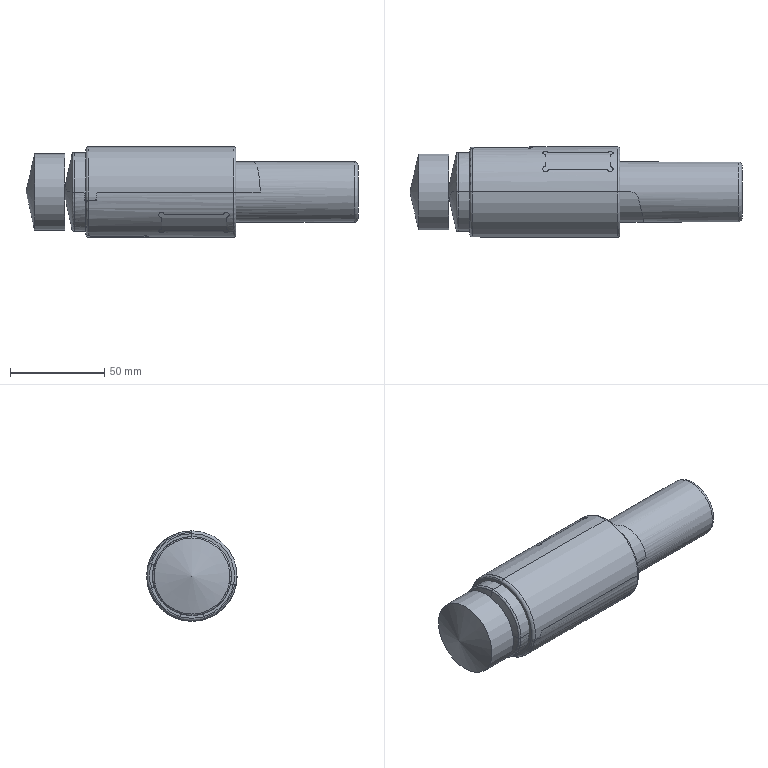NC program | NX | posted with a generic post | part box 176.413 x 48 x 48 mm
Lines 1 to 1741 of 71815:
N10 G17 G21 G94 G90
(FLOOR_WALL , TOOL : D16R0.8)
N12 T16 M6
N14 G54
N16 G17 G0 G90 X-98.197 Y-17.836 S2000 M3
N18 G43 Z30.115 H16
N20 Z24.006
N22 G94 G1 Z22.506 F1000.
N24 X-103.22 Y-9.136
N26 G3 X-104.606 Y-8.336 R1.6
N28 G1 X-143.133 F2000.
N30 G2 X-143.615 Y-8.1 R0.67
N32 G1 X-65.61
N34 X-65.895 Y-8.32
N36 X-66. Y-8.336
N38 X-104.606
N40 G3 X-105.992 Y-9.136 R1.6
N42 G1 X-111.015 Y-17.836
N44 Z24.006
N46 G0 X-98.223 Y-18.479 Z23.757
N48 G1 Z22.257 F1000.
N50 X-103.246 Y-9.779
N52 G3 X-104.632 Y-8.979 R1.6
N54 G1 X-143.142 F2000.
N56 G2 X-144.048 Y-8.1 R1.265
N58 G1 X-65.276
N60 X-65.559 Y-8.702
N62 X-65.618 Y-8.774
N64 X-65.768 Y-8.906
N66 X-65.905 Y-8.967
N68 X-66. Y-8.979
N70 X-104.632
N72 G3 X-106.017 Y-9.779 R1.6
N74 G1 X-111.04 Y-18.479
N76 Z23.757
N78 G0 X-98.843 Y-19.073 Z23.508
N80 G1 Z22.008 F1000.
N82 X-103.866 Y-10.373
N84 G3 X-105.252 Y-9.573 R1.6
N86 G1 X-143.133 F2000.
N88 X-143.218 Y-9.567
N90 X-143.587 Y-9.395
N92 X-143.969 Y-8.916
N94 X-144.131 Y-8.575
N96 X-144.292 Y-8.1
N98 X-65.088
N100 G2 X-65.494 Y-9.248 R3.11
N102 G1 X-65.705 Y-9.461
N104 X-65.842 Y-9.541
N106 X-65.98 Y-9.573
N108 X-105.252
N110 G3 X-106.638 Y-10.373 R1.6
N112 G1 X-111.661 Y-19.073
N114 Z23.508
N116 G0 X-99.004 Y-19.626 Z23.259
N118 G1 Z21.759 F1000.
N120 X-104.027 Y-10.926
N122 G3 X-105.413 Y-10.126 R1.6
N124 G1 X-143.156 F2000.
N126 G2 X-143.924 Y-9.579 R1.015
N128 G1 X-144.104 Y-9.249
N130 X-144.259 Y-8.852
N132 X-144.447 Y-8.1
N134 X-65.
N136 G2 X-65.352 Y-9.578 R4.236
N138 X-66. Y-10.126 R0.876
N140 G1 X-105.413
N142 G3 X-106.798 Y-10.926 R1.6
N144 G1 X-111.821 Y-19.626
N146 Z23.259
N148 G0 X-99.265 Y-20.145 Z23.01
N150 G1 Z21.51 F1000.
N152 X-104.288 Y-11.445
N154 G3 X-105.674 Y-10.645 R1.6
N156 G1 X-143.133 F2000.
N158 X-143.313 Y-10.62
N160 X-143.589 Y-10.484
N162 X-143.774 Y-10.316
N164 G2 X-144.546 Y-8.1 R4.023
N166 G1 X-64.999
N168 X-65.027 Y-8.901
N170 G2 X-65.333 Y-10.089 R3.297
N172 G1 X-65.705 Y-10.544
N174 X-66. Y-10.645
N176 X-105.674
N178 G3 X-107.059 Y-11.445 R1.6
N180 G1 X-112.082 Y-20.145
N182 Z23.01
N184 G0 X-98.654 Y-20.634 Z22.761
N186 G1 Z21.261 F1000.
N188 X-103.677 Y-11.934
N190 G3 X-105.063 Y-11.134 R1.6
N192 G1 X-143.133 F2000.
N194 G2 X-144.126 Y-10.298 R1.212
N196 G1 X-144.302 Y-9.879
N198 G2 X-144.631 Y-8.1 R6.287
N200 G1 X-65.
N202 X-65.03 Y-9.501
N204 G2 X-65.367 Y-10.657 R2.686
N206 G1 X-65.72 Y-11.048
N208 X-66. Y-11.134
N210 X-105.063
N212 G3 X-106.448 Y-11.934 R1.6
N214 G1 X-111.471 Y-20.634
N216 Z22.761
N218 G0 X-98.554 Y-21.097 Z22.512
N220 G1 Z21.012 F1000.
N222 X-103.577 Y-12.397
N224 G3 X-104.963 Y-11.597 R1.6
N226 G1 X-143.133 F2000.
N228 G2 X-144.092 Y-10.862 R1.1
N230 G1 X-144.31 Y-10.391
N232 G2 X-144.633 Y-8.206 R6.418
N234 G1 Y-8.1
N236 X-65.
N238 Y-8.935
N240 X-64.999 Y-9.628
N242 G2 X-65.276 Y-10.985 R3.254
N244 X-65.93 Y-11.592 R1.015
N246 G1 X-66. Y-11.597
N248 X-104.963
N250 G3 X-106.348 Y-12.397 R1.6
N252 G1 X-111.371 Y-21.097
N254 Z22.512
N256 G0 X-100.012 Y-21.537 Z22.263
N258 G1 Z20.763 F1000.
N260 X-105.035 Y-12.837
N262 G3 X-106.42 Y-12.037 R1.6
N264 G1 X-143.187 Y-12.035 F2000.
N266 G2 X-144.11 Y-11.299 R1.22
N268 G1 X-144.328 Y-10.831
N270 G2 X-144.57 Y-9.816 R6.02
N272 G1 X-144.823 Y-8.1
N274 X-65.
N276 Y-9.765
N278 Y-10.121
N280 G2 X-65.33 Y-11.539 R3.11
N282 G1 X-65.696 Y-11.942
N284 X-66. Y-12.037
N286 X-106.42
N288 G3 X-107.806 Y-12.837 R1.6
N290 G1 X-112.829 Y-21.537
N292 Z22.263
N294 G0 X-97.913 Y-21.956 Z22.014
N296 G1 Z20.514 F1000.
N298 X-102.936 Y-13.256
N300 G3 X-104.322 Y-12.456 R1.6
N302 G1 X-143.301 F2000.
N304 G2 X-143.56 Y-12.363 R0.818
N306 G1 X-143.863 Y-12.087
N308 X-144.058 Y-11.83
N310 X-144.287 Y-11.403
N312 G2 X-144.509 Y-10.656 R5.376
N314 G1 X-145.07 Y-8.1
N316 X-65.
N318 X-65.019 Y-10.828
N320 X-65.106 Y-11.423
N322 G2 X-65.442 Y-12.144 R1.812
N324 G1 X-65.802 Y-12.418
N326 X-65.96 Y-12.455
N328 X-104.322 Y-12.456
N330 G3 X-105.707 Y-13.256 R1.6
N332 G1 X-110.73 Y-21.956
N334 Z22.014
N336 G0 X-100.502 Y-22.357 Z21.765
N338 G1 Z20.265 F1000.
N340 X-105.525 Y-13.657
N342 G3 X-106.91 Y-12.857 R1.6
N344 G1 X-143.159 F2000.
N346 G2 X-144.09 Y-12.202 R1.193
N348 G1 X-144.316 Y-11.769
N350 G2 X-144.456 Y-11.33 R5.168
N352 G1 X-145.325 Y-8.1
N354 X-65.
N356 Y-10.582
N358 X-64.998 Y-11.043
N360 G2 X-65.345 Y-12.421 R2.704
N362 G1 X-65.542 Y-12.649
N364 X-65.693 Y-12.767
N366 X-66. Y-12.857
N368 X-106.91
N370 G3 X-108.296 Y-13.657 R1.6
N372 G1 X-113.319 Y-22.357
N374 Z21.765
N376 G0 X-100.642 Y-22.742 Z21.516
N378 G1 Z20.016 F1000.
N380 X-105.665 Y-14.042
N382 G3 X-107.051 Y-13.242 R1.6
N384 G1 X-143.133 F2000.
N386 G2 X-144.023 Y-12.704 R1.1
N388 G1 X-144.269 Y-12.31
N390 G2 X-144.441 Y-11.862 R4.065
N392 G1 X-145.637 Y-8.1
N394 X-65.
N396 X-64.998 Y-11.043
N398 X-65. Y-11.226
N400 Y-11.506
N402 G2 X-65.249 Y-12.648 R2.895
N404 G1 X-65.454 Y-12.945
N406 X-65.604 Y-13.093
N408 X-65.941 Y-13.239
N410 X-66. Y-13.242
N412 X-107.051
N414 G3 X-108.437 Y-14.042 R1.6
N416 G1 X-113.46 Y-22.742
N418 Z21.516
N420 G0 X-101.061 Y-23.111 Z21.267
N422 G1 Z19.767 F1000.
N424 X-106.084 Y-14.411
N426 G3 X-107.469 Y-13.611 R1.6
N428 G1 X-143.133 F2000.
N430 G2 X-144.197 Y-12.84 R1.247
N432 X-144.407 Y-12.353 R3.996
N434 G1 X-145.911 Y-8.1
N436 X-65.
N438 X-65.03 Y-12.224
N440 X-65.133 Y-12.767
N442 G2 X-65.457 Y-13.363 R1.509
N444 G1 X-65.855 Y-13.592
N446 X-66. Y-13.611
N448 X-107.469
N450 G3 X-108.855 Y-14.411 R1.6
N452 G1 X-113.878 Y-23.111
N454 Z21.267
N456 G0 X-101.143 Y-23.465 Z21.019
N458 G1 Z19.519 F1000.
N460 X-106.166 Y-14.765
N462 G3 X-107.552 Y-13.965 R1.6
N464 G1 X-143.133 F2000.
N466 X-143.345 Y-13.939
N468 X-143.718 Y-13.76
N470 X-143.92 Y-13.578
N472 X-144.118 Y-13.322
N474 X-144.359 Y-12.876
N476 X-146.143 Y-8.137
N478 X-146.598 Y-8.1
N480 X-65.
N482 X-65.032 Y-12.714
N484 G2 X-65.321 Y-13.545 R1.971
N486 G1 X-65.575 Y-13.802
N488 X-65.637 Y-13.847
N490 X-66. Y-13.965
N492 X-107.552
N494 G3 X-108.937 Y-14.765 R1.6
N496 G1 X-113.96 Y-23.465
N498 Z21.019
N500 G0 X-98.202 Y-23.807 Z20.77
N502 G1 Z19.27 F1000.
N504 X-103.225 Y-15.107
N506 G3 X-104.611 Y-14.307 R1.6
N508 G1 X-143.133 F2000.
N510 G2 X-144.167 Y-13.629 R1.292
N512 X-144.361 Y-13.235 R3.566
N514 G1 X-146.294 Y-8.597
N516 X-147.856 Y-8.512
N518 Y-8.1
N520 X-65.
N522 X-65.026 Y-12.971
N524 G2 X-65.637 Y-14.192 R1.633
N526 G1 X-66. Y-14.307
N528 X-104.611
N530 G3 X-105.997 Y-15.107 R1.6
N532 G1 X-111.02 Y-23.807
N534 Z20.77
N536 G0 X-101.11 Y-24.136 Z20.521
N538 G1 Z19.021 F1000.
N540 X-106.133 Y-15.436
N542 G3 X-107.518 Y-14.636 R1.6
N544 G1 X-143.133 F2000.
N546 G2 X-144.099 Y-14.051 R1.197
N548 G1 X-144.353 Y-13.627
N550 X-146.38 Y-9.003
N552 X-147.856 Y-8.969
N554 Y-8.1
N556 X-65.
N558 X-65.032 Y-13.457
N560 G2 X-65.321 Y-14.237 R1.791
N562 G1 X-65.578 Y-14.483
N564 X-65.651 Y-14.533
N566 X-66. Y-14.636
N568 X-107.518
N570 G3 X-108.904 Y-15.436 R1.6
N572 G1 X-113.927 Y-24.136
N574 Z20.521
N576 G0 X-97.817 Y-24.454 Z20.272
N578 G1 Z18.772 F1000.
N580 X-102.84 Y-15.754
N582 G3 X-104.225 Y-14.954 R1.6
N584 G1 X-143.133 F2000.
N586 G2 X-144.127 Y-14.342 R1.2
N588 G1 X-144.406 Y-13.858
N590 X-146.44 Y-9.44
N592 X-147.856 Y-9.432
N594 Y-8.1
N596 X-65.
N598 X-65.023 Y-13.658
N600 G2 X-65.653 Y-14.854 R1.529
N602 G1 X-66. Y-14.954
N604 X-104.225
N606 G3 X-105.611 Y-15.754 R1.6
N608 G1 X-110.634 Y-24.454
N610 Z20.272
N612 G0 X-100.993 Y-24.761 Z20.023
N614 G1 Z18.523 F1000.
N616 X-106.016 Y-16.061
N618 G3 X-107.402 Y-15.261 R1.6
N620 G1 X-143.206 Y-15.259 F2000.
N622 X-143.668 Y-15.106
N624 X-143.877 Y-14.949
N626 X-144.07 Y-14.739
N628 X-144.335 Y-14.334
N630 X-146.479 Y-9.895
N632 X-147.856
N634 Y-8.1
N636 X-65.
N638 X-65.023 Y-14.113
N640 G2 X-65.292 Y-14.835 R1.815
N642 G1 X-65.542 Y-15.087
N644 X-65.622 Y-15.145
N646 X-65.803 Y-15.23
N648 X-65.977 Y-15.261
N650 X-107.402
N652 G3 X-108.788 Y-16.061 R1.6
N654 G1 X-113.81 Y-24.761
N656 Z20.023
N658 G0 X-97.282 Y-25.059 Z19.774
N660 G1 Z18.274 F1000.
N662 X-102.304 Y-16.359
N664 G3 X-103.69 Y-15.559 R1.6
N666 G1 X-143.133 F2000.
N668 X-143.241 Y-15.553
N670 X-143.458 Y-15.504
N672 X-143.56 Y-15.463
N674 X-144.009 Y-15.12
N676 X-144.305 Y-14.718
N678 X-146.411 Y-10.549
N680 X-147.856 Y-10.484
N682 Y-8.1
N684 X-65.
N686 X-65.023 Y-14.315
N688 G2 X-65.68 Y-15.477 R1.424
N690 G1 X-66. Y-15.559
N692 X-103.69
N694 G3 X-105.076 Y-16.359 R1.6
N696 G1 X-110.099 Y-25.059
N698 Z19.774
N700 G0 X-97.018 Y-25.346 Z19.525
N702 G1 Z18.025 F1000.
N704 X-102.041 Y-16.646
N706 G3 X-103.427 Y-15.846 R1.6
N708 G1 X-143.133 F2000.
N710 G2 X-144.236 Y-15.139 R1.354
N712 G1 X-144.29 Y-15.04
N714 X-146.368 Y-11.084
N716 X-147.856 Y-10.982
N718 Y-8.1
N720 X-65.
N722 Y-14.287
N724 G2 X-65.611 Y-15.727 R1.652
N726 G1 X-65.684 Y-15.769
N728 X-65.843 Y-15.828
N730 X-66. Y-15.846
N732 X-103.427
N734 G3 X-104.813 Y-16.646 R1.6
N736 G1 X-109.836 Y-25.346
N738 Z19.525
N740 G0 X-100.846 Y-25.625 Z19.276
N742 G1 Z17.776 F1000.
N744 X-105.869 Y-16.925
N746 G3 X-107.255 Y-16.125 R1.6
N748 G1 X-143.133 F2000.
N750 G2 X-144.16 Y-15.514 R1.268
N752 G1 X-146.715 Y-11.181
N754 X-147.856
N756 Y-8.1
N758 X-65.
N760 Y-14.556
N762 Y-14.757
N764 G2 X-65.26 Y-15.676 R1.72
N766 G1 X-65.514 Y-15.937
N768 X-65.6 Y-16.
N770 X-65.765 Y-16.084
N772 X-65.943 Y-16.123
N774 X-107.255 Y-16.125
N776 G3 X-108.64 Y-16.925 R1.6
N778 G1 X-113.663 Y-25.625
N780 Z19.276
N782 G0 X-96.821 Y-25.895 Z19.027
N784 G1 Z17.527 F1000.
N786 X-101.844 Y-17.195
N788 G3 X-103.23 Y-16.395 R1.6
N790 G1 X-143.133 F2000.
N792 G2 X-144.315 Y-15.589 R1.416
N794 G1 X-146.577 Y-11.568
N796 X-147.856
N798 Y-8.1
N800 X-65.
N802 X-65.023 Y-15.218
N804 G2 X-65.879 Y-16.385 R1.309
N806 G1 X-66. Y-16.395
N808 X-103.23
N810 G3 X-104.616 Y-17.195 R1.6
N812 G1 X-109.639 Y-25.895
N814 Z19.027
N816 G0 X-96.475 Y-26.158 Z18.778
N818 G1 Z17.278 F1000.
N820 X-101.498 Y-17.458
N822 G3 X-102.884 Y-16.658 R1.6
N824 G1 X-143.145 Y-16.657 F2000.
N826 G2 X-144.078 Y-16.172 R1.219
N828 G1 X-144.395 Y-15.724
N830 X-146.402 Y-12.223
N832 X-147.856 Y-12.13
N834 Y-8.1
N836 X-65.
N838 Y-15.181
N840 G2 X-65.824 Y-16.635 R1.414
N842 G1 X-66. Y-16.658
N844 X-102.884
N846 G3 X-104.27 Y-17.458 R1.6
N848 G1 X-109.293 Y-26.158
N850 Z18.778
N852 G0 X-96.479 Y-26.412 Z18.529
N854 G1 Z17.029 F1000.
N856 X-101.502 Y-17.712
N858 G3 X-102.888 Y-16.912 R1.6
N860 G1 X-143.133 F2000.
N862 X-143.283 Y-16.901
N864 X-143.776 Y-16.706
N866 X-143.986 Y-16.532
N868 X-144.295 Y-16.166
N870 X-146.598 Y-12.289
N872 X-147.856
N874 Y-8.1
N876 X-65.
N878 Y-15.46
N880 G2 X-65.753 Y-16.868 R1.47
N882 G1 X-65.935 Y-16.909
N884 X-66. Y-16.912
N886 X-102.888
N888 G3 X-104.274 Y-17.712 R1.6
N890 G1 X-109.297 Y-26.412
N892 Z18.529
N894 G0 X-96.414 Y-26.659 Z18.28
N896 G1 Z16.78 F1000.
N898 X-101.437 Y-17.959
N900 G3 X-102.823 Y-17.159 R1.6
N902 G1 X-143.133 F2000.
N904 X-143.362 Y-17.134
N906 X-143.813 Y-16.931
N908 X-143.887 Y-16.874
N910 X-144.089 Y-16.674
N912 X-146.958 Y-12.627
N914 X-147.856
N916 Y-8.1
N918 X-65.
N920 Y-15.73
N922 X-65.022 Y-16.036
N924 X-65.078 Y-16.292
N926 X-65.174 Y-16.542
N928 X-65.517 Y-16.985
N930 X-65.87 Y-17.147
N932 X-66. Y-17.159
N934 X-102.823
N936 G3 X-104.209 Y-17.959 R1.6
N938 G1 X-109.232 Y-26.659
N940 Z18.28
N942 G0 X-96.072 Y-26.899 Z18.031
N944 G1 Z16.531 F1000.
N946 X-101.095 Y-18.199
N948 G3 X-102.481 Y-17.399 R1.6
N950 G1 X-143.198 Y-17.397 F2000.
N952 X-143.428 Y-17.359
N954 X-143.561 Y-17.313
N956 X-143.999 Y-17.017
N958 X-144.31 Y-16.651
N960 X-146.507 Y-13.102
N962 X-147.856 Y-13.056
N964 Y-8.1
N966 X-65.
N968 Y-15.991
N970 G2 X-65.822 Y-17.377 R1.388
N972 G1 X-66. Y-17.399
N974 X-102.481
N976 G3 X-103.866 Y-18.199 R1.6
N978 G1 X-108.889 Y-26.899
N980 Z18.031
N982 G0 X-96.078 Y-27.132 Z17.782
N984 G1 Z16.282 F1000.
N986 X-101.101 Y-18.432
N988 G3 X-102.487 Y-17.632 R1.6
N990 G1 X-143.133 F2000.
N992 X-143.307 Y-17.618
N994 X-143.536 Y-17.557
N996 X-143.66 Y-17.502
N998 X-144.112 Y-17.134
N1000 X-146.846 Y-13.262
N1002 X-147.856
N1004 Y-8.1
N1006 X-65.
N1008 Y-16.245
N1010 G2 X-65.761 Y-17.593 R1.367
N1012 G1 X-65.948 Y-17.63
N1014 X-102.487 Y-17.632
N1016 G3 X-103.872 Y-18.432 R1.6
N1018 G1 X-108.895 Y-27.132
N1020 Z17.782
N1022 G0 X-95.773 Y-27.359 Z17.533
N1024 G1 Z16.033 F1000.
N1026 X-100.796 Y-18.659
N1028 G3 X-102.182 Y-17.859 R1.6
N1030 G1 X-143.309 Y-17.845 F2000.
N1032 G2 X-144.245 Y-17.19 R1.386
N1034 G1 X-146.243 Y-13.562
N1036 X-147.856
N1038 Y-8.1
N1040 X-65.
N1042 Y-16.491
N1044 X-65.022 Y-16.783
N1046 X-65.095 Y-17.079
N1048 X-65.198 Y-17.315
N1050 X-65.546 Y-17.712
N1052 X-65.872 Y-17.848
N1054 X-66. Y-17.859
N1056 X-102.182
N1058 G3 X-103.568 Y-18.659 R1.6
N1060 G1 X-108.591 Y-27.359
N1062 Z17.533
N1064 G0 X-95.813 Y-27.579 Z17.284
N1066 G1 Z15.784 F1000.
N1068 X-100.836 Y-18.879
N1070 G3 X-102.221 Y-18.079 R1.6
N1072 G1 X-143.133 F2000.
N1074 X-143.259 Y-18.072
N1076 X-143.686 Y-17.939
N1078 X-143.905 Y-17.794
N1080 X-144.096 Y-17.612
N1082 X-146.903 Y-13.851
N1084 X-147.856
N1086 Y-8.1
N1088 X-65.
N1090 Y-16.729
N1092 G2 X-66. Y-18.079 R1.22
N1094 G1 X-102.221
N1096 G3 X-103.607 Y-18.879 R1.6
N1098 G1 X-108.63 Y-27.579
N1100 Z17.284
N1102 G0 X-95.577 Y-27.794 Z17.035
N1104 G1 Z15.535 F1000.
N1106 X-100.6 Y-19.094
N1108 G3 X-101.986 Y-18.294 R1.6
N1110 G1 X-143.133 F2000.
N1112 X-143.368 Y-18.269
N1114 X-143.765 Y-18.11
N1116 X-143.98 Y-17.948
N1118 X-144.171 Y-17.743
N1120 X-146.55 Y-14.13
N1122 X-147.856
N1124 Y-8.1
N1126 X-65.
N1128 Y-16.96
N1130 G2 X-65.975 Y-18.293 R1.185
N1132 G1 X-101.986 Y-18.294
N1134 G3 X-103.372 Y-19.094 R1.6
N1136 G1 X-108.395 Y-27.794
N1138 Z17.035
N1140 G0 X-95.362 Y-28.002 Z16.786
N1142 G1 Z15.286 F1000.
N1144 X-100.385 Y-19.302
N1146 G3 X-101.771 Y-18.502 R1.6
N1148 G1 X-143.133 F2000.
N1150 X-143.371 Y-18.478
N1152 X-143.849 Y-18.266
N1154 X-144.059 Y-18.086
N1156 X-144.246 Y-17.856
N1158 X-146.226 Y-14.399
N1160 X-147.856
N1162 Y-8.1
N1164 X-65.
N1166 Y-17.185
N1168 G2 X-66. Y-18.502 R1.188
N1170 G1 X-101.771
N1172 G3 X-103.157 Y-19.302 R1.6
N1174 G1 X-108.179 Y-28.002
N1176 Z16.786
N1178 G0 X-95.354 Y-28.205 Z16.537
N1180 G1 Z15.037 F1000.
N1182 X-100.377 Y-19.505
N1184 G3 X-101.763 Y-18.705 R1.6
N1186 G1 X-143.158 F2000.
N1188 X-143.397 Y-18.675
N1190 X-143.937 Y-18.405
N1192 X-144.139 Y-18.206
N1194 X-146.663 Y-14.659
N1196 X-147.856
N1198 Y-8.1
N1200 X-65.
N1202 X-65.023 Y-17.686
N1204 G2 X-66. Y-18.705 R1.05
N1206 G1 X-101.763
N1208 G3 X-103.149 Y-19.505 R1.6
N1210 G1 X-108.172 Y-28.205
N1212 Z16.537
N1214 G0 X-95.133 Y-28.403 Z16.288
N1216 G1 Z14.788 F1000.
N1218 X-100.156 Y-19.703
N1220 G3 X-101.541 Y-18.903 R1.6
N1222 G1 X-143.202 Y-18.9 F2000.
N1224 X-143.441 Y-18.862
N1226 X-143.595 Y-18.81
N1228 X-144.027 Y-18.526
N1230 X-144.219 Y-18.308
N1232 X-146.299 Y-14.91
N1234 X-147.856
N1236 Y-8.1
N1238 X-65.
N1240 X-65.023 Y-17.892
N1242 G2 X-66. Y-18.903 R1.093
N1244 G1 X-101.541
N1246 G3 X-102.927 Y-19.703 R1.6
N1248 G1 X-107.95 Y-28.403
N1250 Z16.288
N1252 G0 X-95.145 Y-28.595 Z16.039
N1254 G1 Z14.539 F1000.
N1256 X-100.168 Y-19.895
N1258 G3 X-101.553 Y-19.095 R1.6
N1260 G1 X-143.133 F2000.
N1262 X-143.373 Y-19.07
N1264 X-143.781 Y-18.909
N1266 X-143.996 Y-18.75
N1268 X-144.118 Y-18.629
N1270 X-146.758 Y-15.153
N1272 X-147.856
N1274 Y-8.1
N1276 X-65.
N1278 Y-17.821
N1280 G2 X-65.964 Y-19.094 R1.158
N1282 G1 X-101.553 Y-19.095
N1284 G3 X-102.939 Y-19.895 R1.6
N1286 G1 X-107.962 Y-28.595
N1288 Z16.039
N1290 G0 X-95.06 Y-28.782 Z15.79
N1292 G1 Z14.29 F1000.
N1294 X-100.083 Y-20.082
N1296 G3 X-101.469 Y-19.282 R1.6
N1298 G1 X-143.133 F2000.
N1300 G2 X-144.098 Y-18.842 R1.319
N1302 G1 X-146.85 Y-15.388
N1304 X-147.856
N1306 Y-8.1
N1308 X-65.
N1310 Y-18.022
N1312 G2 X-66. Y-19.282 R1.158
N1314 G1 X-101.469
N1316 G3 X-102.854 Y-20.082 R1.6
N1318 G1 X-107.877 Y-28.782
N1320 Z15.79
N1322 G0 X-94.913 Y-28.964 Z15.541
N1324 G1 Z14.041 F1000.
N1326 X-99.936 Y-20.264
N1328 G3 X-101.322 Y-19.464 R1.6
N1330 G1 X-143.174 Y-19.463 F2000.
N1332 G2 X-144.123 Y-19.002 R1.338
N1334 G1 X-146.728 Y-15.615
N1336 X-147.856
N1338 Y-8.1
N1340 X-65.
N1342 Y-18.216
N1344 G2 X-66. Y-19.464 R1.134
N1346 G1 X-101.322
N1348 G3 X-102.707 Y-20.264 R1.6
N1350 G1 X-107.73 Y-28.964
N1352 Z15.541
N1354 G0 X-94.765 Y-29.141 Z15.293
N1356 G1 Z13.793 F1000.
N1358 X-99.788 Y-20.441
N1360 G3 X-101.173 Y-19.641 R1.6
N1362 G1 X-143.133 F2000.
N1364 G2 X-144.156 Y-19.146 R1.352
N1366 G1 X-146.572 Y-15.836
N1368 X-147.856
N1370 Y-8.1
N1372 X-62.231
N1374 X-62.229 Y-8.11
N1376 X-65.
N1378 Y-18.406
N1380 G2 X-66. Y-19.641 R1.133
N1382 G1 X-101.173
N1384 G3 X-102.559 Y-20.441 R1.6
N1386 G1 X-107.582 Y-29.141
N1388 Z15.293
N1390 G0 X-94.8 Y-29.313 Z15.044
N1392 G1 Z13.544 F1000.
N1394 X-99.823 Y-20.613
N1396 G3 X-101.209 Y-19.813 R1.6
N1398 G1 X-143.133 F2000.
N1400 X-143.378 Y-19.789
N1402 X-143.807 Y-19.619
N1404 X-144.024 Y-19.457
N1406 X-144.21 Y-19.259
N1408 X-146.342 Y-16.049
N1410 X-147.856
N1412 Y-8.1
N1414 X-62.231
N1416 X-62.131 Y-8.519
N1418 X-65.
N1420 Y-18.59
N1422 G2 X-66. Y-19.813 R1.154
N1424 G1 X-101.209
N1426 G3 X-102.595 Y-20.613 R1.6
N1428 G1 X-107.618 Y-29.313
N1430 Z15.044
N1432 G0 X-95.063 Y-29.481 Z14.795
N1434 G1 Z13.295 F1000.
N1436 X-100.086 Y-20.781
N1438 G3 X-101.472 Y-19.981 R1.6
N1440 G1 X-143.133 F2000.
N1442 X-143.379 Y-19.957
N1444 X-143.871 Y-19.748
N1446 X-144.083 Y-19.573
N1448 X-146.909 Y-16.256
N1450 X-147.856
N1452 Y-8.1
N1454 X-62.231
N1456 X-62.038 Y-8.902
N1458 X-65.
N1460 X-65.001 Y-18.818
N1462 G2 X-66. Y-19.981 R1.129
N1464 G1 X-101.472
N1466 G3 X-102.858 Y-20.781 R1.6
N1468 G1 X-107.88 Y-29.481
N1470 Z14.795
N1472 G0 X-95.057 Y-29.645 Z14.546
N1474 G1 Z13.046 F1000.
N1476 X-100.08 Y-20.945
N1478 G3 X-101.466 Y-20.145 R1.6
N1480 G1 X-143.212 Y-20.142 F2000.
N1482 G2 X-144.142 Y-19.678 R1.373
N1484 G1 X-146.622 Y-16.456
N1486 X-147.856
N1488 Y-8.1
N1490 X-62.231
N1492 X-61.951 Y-9.263
N1494 X-65.
N1496 X-65.024 Y-19.205
N1498 G2 X-66. Y-20.145 R1.059
N1500 G1 X-101.466
N1502 G3 X-102.851 Y-20.945 R1.6
N1504 G1 X-107.874 Y-29.645
N1506 Z14.546
N1508 G0 X-95.055 Y-29.804 Z14.297
N1510 G1 Z12.797 F1000.
N1512 X-100.078 Y-21.104
N1514 G3 X-101.463 Y-20.304 R1.6
N1516 G1 X-143.133 F2000.
N1518 G2 X-144.203 Y-19.772 R1.383
N1520 G1 X-146.354 Y-16.651
N1522 X-147.856
N1524 Y-8.1
N1526 X-62.231
N1528 X-61.869 Y-9.604
N1530 X-65.
N1532 Y-19.111
N1534 G2 X-66. Y-20.304 R1.124
N1536 G1 X-101.463
N1538 G3 X-102.849 Y-21.104 R1.6
N1540 G1 X-107.872 Y-29.804
N1542 Z14.297
N1544 G0 X-95.297 Y-29.959 Z14.048
N1546 G1 Z12.548 F1000.
N1548 X-100.32 Y-21.259
N1550 G3 X-101.706 Y-20.459 R1.6
N1552 G1 X-143.133 F2000.
N1554 G2 X-144.075 Y-20.067 R1.358
N1556 G1 X-146.914 Y-16.839
N1558 X-147.856
N1560 Y-8.1
N1562 X-62.231
N1564 X-61.792 Y-9.927
N1566 X-65.
N1568 Y-19.276
N1570 G2 X-66. Y-20.459 R1.086
N1572 G1 X-101.706
N1574 G3 X-103.092 Y-21.259 R1.6
N1576 G1 X-108.115 Y-29.959
N1578 Z14.048
N1580 G0 X-95.258 Y-30.109 Z13.799
N1582 G1 Z12.299 F1000.
N1584 X-100.281 Y-21.409
N1586 G3 X-101.667 Y-20.609 R1.6
N1588 G1 X-143.133 F2000.
N1590 G2 X-144.147 Y-20.149 R1.382
N1592 G1 X-146.586 Y-17.022
N1594 X-147.856
N1596 Y-8.1
N1598 X-62.231
N1600 X-61.718 Y-10.234
N1602 X-65.
N1604 Y-19.436
N1606 G2 X-65.966 Y-20.609 R1.091
N1608 G1 X-101.667
N1610 G3 X-103.052 Y-21.409 R1.6
N1612 G1 X-108.075 Y-30.109
N1614 Z13.799
N1616 G0 X-95.23 Y-30.256 Z13.55
N1618 G1 Z12.05 F1000.
N1620 X-100.253 Y-21.556
N1622 G3 X-101.638 Y-20.756 R1.6
N1624 G1 X-143.133 F2000.
N1626 G2 X-144.218 Y-20.217 R1.4
N1628 G1 X-146.286 Y-17.199
N1630 X-147.856
N1632 Y-8.1
N1634 X-62.231
N1636 X-61.648 Y-10.526
N1638 X-65.
N1640 Y-19.591
N1642 G2 X-66. Y-20.756 R1.088
N1644 G1 X-101.638
N1646 G3 X-103.024 Y-21.556 R1.6
N1648 G1 X-108.047 Y-30.256
N1650 Z13.55
N1652 G0 X-95.357 Y-30.398 Z13.301
N1654 G1 Z11.801 F1000.
N1656 X-100.38 Y-21.698
N1658 G3 X-101.766 Y-20.898 R1.6
N1660 G1 X-143.133 F2000.
N1662 G2 X-144.158 Y-20.432 R1.389
N1664 G1 X-146.53 Y-17.371
N1666 X-147.856
N1668 Y-8.102
N1670 X-62.231
N1672 X-61.581 Y-10.805
N1674 X-65.
N1676 Y-19.742
N1678 G2 X-66. Y-20.898 R1.106
N1680 G1 X-101.766
N1682 G3 X-103.152 Y-21.698 R1.6
N1684 G1 X-108.175 Y-30.398
N1686 Z13.301
N1688 G0 X-95.386 Y-30.537 Z13.052
N1690 G1 Z11.552 F1000.
N1692 X-100.409 Y-21.837
N1694 G3 X-101.795 Y-21.037 R1.6
N1696 G1 X-143.133 F2000.
N1698 G2 X-144.176 Y-20.555 R1.398
N1700 G1 X-146.454 Y-17.537
N1702 X-147.856
N1704 Y-8.108
N1706 X-62.229
N1708 X-61.517 Y-11.07
N1710 X-65.
N1712 Y-19.889
N1714 G2 X-66. Y-21.037 R1.102
N1716 G1 X-101.795
N1718 G3 X-103.181 Y-21.837 R1.6
N1720 G1 X-108.204 Y-30.537
N1722 Z13.052
N1724 G0 X-95.408 Y-30.672 Z12.803
N1726 G1 Z11.303 F1000.
N1728 X-100.431 Y-21.972
N1730 G3 X-101.816 Y-21.172 R1.6
N1732 G1 X-143.133 F2000.
N1734 G2 X-144.198 Y-20.668 R1.401
N1736 G1 X-146.362 Y-17.699
N1738 X-147.856
N1740 Y-8.12
N1742 X-62.226
N1744 X-61.456 Y-11.324
N1746 X-65.
N1748 Y-20.031
N1750 G2 X-66. Y-21.172 R1.099
N1752 G1 X-101.816
N1754 G3 X-103.202 Y-21.972 R1.6
N1756 G1 X-108.225 Y-30.672
N1758 Z12.803
N1760 G0 X-95.669 Y-30.803 Z12.554
N1762 G1 Z11.054 F1000.
N1764 X-100.692 Y-22.103
N1766 G3 X-102.078 Y-21.303 R1.6
N1768 G1 X-143.133 F2000.
N1770 G2 X-144.054 Y-20.946 R1.385
N1772 G1 X-147.031 Y-17.855
N1774 X-147.856
N1776 Y-8.137
N1778 X-62.222
N1780 X-61.397 Y-11.568
N1782 X-65.
N1784 Y-20.169
N1786 G2 X-66. Y-21.303 R1.072
N1788 G1 X-102.078
N1790 G3 X-103.464 Y-22.103 R1.6
N1792 G1 X-108.487 Y-30.803
N1794 Z12.554
N1796 G0 X-95.644 Y-30.93 Z12.305
N1798 G1 Z10.805 F1000.
N1800 X-100.667 Y-22.23
N1802 G3 X-102.053 Y-21.43 R1.6
N1804 G1 X-143.133 F2000.
N1806 G2 X-144.094 Y-21.039 R1.397
N1808 G1 X-146.83 Y-18.007
N1810 X-147.856
N1812 Y-8.16
N1814 X-62.217
N1816 X-61.341 Y-11.8
N1818 X-65.
N1820 Y-20.304
N1822 G2 X-65.951 Y-21.429 R1.058
N1824 G1 X-102.053 Y-21.43
N1826 G3 X-103.439 Y-22.23 R1.6
N1828 G1 X-108.462 Y-30.93
N1830 Z12.305
N1832 G0 X-95.622 Y-31.054 Z12.056
N1834 G1 Z10.556 F1000.
N1836 X-100.645 Y-22.354
N1838 G3 X-102.031 Y-21.554 R1.6
N1840 G1 X-143.133 F2000.
N1842 G2 X-144.135 Y-21.125 R1.409
N1844 G1 X-146.638 Y-18.154
N1846 X-147.856
N1848 Y-8.187
N1850 X-62.21
N1852 X-61.288 Y-12.024
N1854 X-65.
N1856 Y-20.434
N1858 G2 X-66. Y-21.554 R1.054
N1860 G1 X-102.031
N1862 G3 X-103.416 Y-22.354 R1.6
N1864 G1 X-108.439 Y-31.054
N1866 Z12.056
N1868 G0 X-95.602 Y-31.174 Z11.807
N1870 G1 Z10.307 F1000.
N1872 X-100.625 Y-22.474
N1874 G3 X-102.011 Y-21.674 R1.6
N1876 G1 X-143.133 F2000.
N1878 G2 X-144.177 Y-21.204 R1.42
N1880 G1 X-146.454 Y-18.297
N1882 X-147.856
N1884 Y-8.22
N1886 X-62.202
N1888 X-61.236 Y-12.238
N1890 X-65.
N1892 Y-20.561
N1894 G2 X-66. Y-21.674 R1.067
N1896 G1 X-102.011
N1898 G3 X-103.396 Y-22.474 R1.6
N1900 G1 X-108.419 Y-31.174
N1902 Z11.807
N1904 G0 X-95.585 Y-31.291 Z11.558
N1906 G1 Z10.058 F1000.
N1908 X-100.608 Y-22.591
N1910 G3 X-101.993 Y-21.791 R1.6
N1912 G1 X-143.133 F2000.
N1914 X-143.389 Y-21.766
N1916 X-143.858 Y-21.585
N1918 X-144.021 Y-21.47
N1920 X-144.22 Y-21.277
N1922 X-146.279 Y-18.435
N1924 X-147.856
N1926 Y-8.258
N1928 X-62.193
N1930 X-61.187 Y-12.443
N1932 X-65.
N1934 X-65.003 Y-20.766
N1936 G2 X-66. Y-21.791 R1.045
N1938 G1 X-101.993
N1940 G3 X-103.379 Y-22.591 R1.6
N1942 G1 X-108.402 Y-31.291
N1944 Z11.558
N1946 G0 X-95.817 Y-31.404 Z11.309
N1948 G1 Z9.809 F1000.
N1950 X-100.84 Y-22.704
N1952 G3 X-102.225 Y-21.904 R1.6
N1954 G1 X-143.133 F2000.
N1956 X-143.39 Y-21.88
N1958 X-143.905 Y-21.669
N1960 X-144.07 Y-21.543
N1962 X-146.897 Y-18.568
N1964 X-147.856
N1966 Y-8.302
N1968 X-62.183
N1970 X-61.139 Y-12.64
N1972 X-65.
N1974 X-65.002 Y-20.864
N1976 G2 X-66. Y-21.904 R1.046
N1978 G1 X-102.225
N1980 G3 X-103.611 Y-22.704 R1.6
N1982 G1 X-108.634 Y-31.404
N1984 Z11.309
N1986 G0 X-95.772 Y-31.514 Z11.06
N1988 G1 Z9.56 F1000.
N1990 X-100.795 Y-22.814
N1992 G3 X-102.18 Y-22.014 R1.6
N1994 G1 X-143.133 F2000.
N1996 X-143.391 Y-21.989
N1998 X-143.954 Y-21.747
N2000 X-144.12 Y-21.609
N2002 X-146.667 Y-18.698
N2004 X-147.856
N2006 Y-8.351
N2008 X-62.171
N2010 X-61.094 Y-12.83
N2012 X-65.
N2014 X-65.001 Y-20.957
N2016 G2 X-66. Y-22.014 R1.046
N2018 G1 X-102.18
N2020 G3 X-103.566 Y-22.814 R1.6
N2022 G1 X-108.589 Y-31.514
N2024 Z11.06
N2026 G0 X-95.733 Y-31.62 Z10.811
N2028 G1 Z9.311 F1000.
N2030 X-100.755 Y-22.92
N2032 G3 X-102.141 Y-22.12 R1.6
N2034 G1 X-143.133 F2000.
N2036 G2 X-144.171 Y-21.667 R1.432
N2038 G1 X-146.451 Y-18.823
N2040 X-147.856
N2042 Y-8.405
N2044 X-62.158
N2046 X-61.05 Y-13.011
N2048 X-65.
N2050 Y-21.043
N2052 G2 X-65.97 Y-22.12 R1.036
N2054 G1 X-102.141
N2056 G3 X-103.527 Y-22.92 R1.6
N2058 G1 X-108.55 Y-31.62
N2060 Z10.811
N2062 G0 X-95.699 Y-31.723 Z10.562
N2064 G1 Z9.062 F1000.
N2066 X-100.722 Y-23.023
N2068 G3 X-102.108 Y-22.223 R1.6
N2070 G1 X-143.193 Y-22.222 F2000.
N2072 G2 X-144.221 Y-21.718 R1.446
N2074 G1 X-146.248 Y-18.944
N2076 X-147.856
N2078 Y-8.465
N2080 X-62.143
N2082 X-61.008 Y-13.186
N2084 X-65.
N2086 Y-21.139
N2088 G2 X-65.942 Y-22.221 R1.038
N2090 G1 X-102.108 Y-22.223
N2092 G3 X-103.493 Y-23.023 R1.6
N2094 G1 X-108.516 Y-31.723
N2096 Z10.562
N2098 G0 X-95.896 Y-31.823 Z10.313
N2100 G1 Z8.813 F1000.
N2102 X-100.919 Y-23.123
N2104 G3 X-102.305 Y-22.323 R1.6
N2106 G1 X-143.133 F2000.
N2108 G2 X-144.107 Y-21.936 R1.432
N2110 G1 X-146.781 Y-19.061
N2112 X-147.856
N2114 Y-8.531
N2116 X-62.128
N2118 X-60.968 Y-13.354
N2120 X-65.
N2122 Y-21.244
N2124 G2 X-66. Y-22.323 R1.034
N2126 G1 X-102.305
N2128 G3 X-103.69 Y-23.123 R1.6
N2130 G1 X-108.713 Y-31.823
N2132 Z10.313
N2134 G0 X-95.772 Y-31.92 Z10.064
N2136 G1 Z8.564 F1000.
N2138 X-100.795 Y-23.22
N2140 G3 X-102.181 Y-22.42 R1.6
N2142 G1 X-143.133 F2000.
N2144 G2 X-144.203 Y-21.939 R1.446
N2146 G1 X-146.317 Y-19.174
N2148 X-147.856
N2150 Y-8.602
N2152 X-62.11
N2154 X-60.929 Y-13.515
N2156 X-65.
N2158 Y-21.346
N2160 G2 X-66. Y-22.42 R1.042
N2162 G1 X-102.181
N2164 G3 X-103.566 Y-23.22 R1.6
N2166 G1 X-108.589 Y-31.92
N2168 Z10.064
N2170 G0 X-95.779 Y-32.013 Z9.816
N2172 G1 Z8.316 F1000.
N2174 X-100.802 Y-23.313
N2176 G3 X-102.187 Y-22.513 R1.6
N2178 G1 X-143.133 F2000.
N2180 G2 X-144.213 Y-22.023 R1.45
N2182 G1 X-146.276 Y-19.283
N2184 X-147.856
N2186 Y-8.68
N2188 X-62.092
N2190 X-60.892 Y-13.669
N2192 X-64.613
N2194 X-65.006 Y-21.558
N2196 G2 X-66. Y-22.513 R1.026
N2198 G1 X-102.187
N2200 G3 X-103.573 Y-23.313 R1.6
N2202 G1 X-108.596 Y-32.013
N2204 Z9.816
N2206 G0 X-96.045 Y-32.104 Z9.567
N2208 G1 Z8.067 F1000.
N2210 X-101.068 Y-23.404
N2212 G3 X-102.453 Y-22.604 R1.6
N2214 G1 X-143.133 F2000.
N2216 X-143.383 Y-22.582
N2218 X-143.638 Y-22.511
N2220 X-143.844 Y-22.414
N2222 X-144.065 Y-22.259
N2224 X-147.006 Y-19.389
N2226 X-147.856
N2228 Y-8.763
N2230 X-62.072
N2232 X-60.856 Y-13.818
N2234 X-64.657
N2236 X-65.004 Y-21.64
N2238 G2 X-66. Y-22.604 R1.026
N2240 G1 X-102.453
N2242 G3 X-103.839 Y-23.404 R1.6
N2244 G1 X-108.862 Y-32.104
N2246 Z9.567
N2248 G0 X-96.073 Y-32.191 Z9.318
N2250 G1 Z7.818 F1000.
N2252 X-101.096 Y-23.491
N2254 G3 X-102.482 Y-22.691 R1.6
N2256 G1 X-143.133 F2000.
N2258 X-143.396 Y-22.667
N2260 X-143.597 Y-22.613
N2262 X-143.828 Y-22.51
N2264 X-144.052 Y-22.358
N2266 X-147.021 Y-19.491
N2268 X-147.856
N2270 Y-8.852
N2272 X-62.05
N2274 X-60.822 Y-13.96
N2276 X-64.705
N2278 X-65.003 Y-21.717
N2280 G2 X-66. Y-22.691 R1.025
N2282 G1 X-102.482
N2284 G3 X-103.868 Y-23.491 R1.6
N2286 G1 X-108.891 Y-32.191
N2288 Z9.318
N2290 G0 X-96.054 Y-32.275 Z9.069
N2292 G1 Z7.569 F1000.
N2294 X-101.077 Y-23.575
N2296 G3 X-102.463 Y-22.775 R1.6
N2298 G1 X-143.149 F2000.
N2300 X-143.412 Y-22.748
N2302 X-143.622 Y-22.689
N2304 X-143.854 Y-22.581
N2306 X-144.076 Y-22.424
N2308 X-146.905 Y-19.589
N2310 X-147.856
N2312 Y-8.948
N2314 X-62.027
N2316 X-60.789 Y-14.097
N2318 X-64.758
N2320 X-65.002 Y-21.79
N2322 G2 X-66. Y-22.775 R1.025
N2324 G1 X-102.463
N2326 G3 X-103.848 Y-23.575 R1.6
N2328 G1 X-108.871 Y-32.275
N2330 Z9.069
N2332 G0 X-96.036 Y-32.357 Z8.82
N2334 G1 Z7.32 F1000.
N2336 X-101.059 Y-23.657
N2338 G3 X-102.445 Y-22.857 R1.6
N2340 G1 X-143.174 Y-22.856 F2000.
N2342 X-143.437 Y-22.824
N2344 X-143.646 Y-22.762
N2346 X-143.88 Y-22.647
N2348 X-144.099 Y-22.486
N2350 X-146.794 Y-19.683
N2352 X-147.856
N2354 Y-9.05
N2356 X-62.003
N2358 X-60.757 Y-14.228
N2360 X-64.817
N2362 X-65.001 Y-21.858
N2364 G2 X-66. Y-22.857 R1.017
N2366 G1 X-102.445
N2368 G3 X-103.83 Y-23.657 R1.6
N2370 G1 X-108.853 Y-32.357
N2372 Z8.82
N2374 G0 X-96.019 Y-32.435 Z8.571
N2376 G1 Z7.071 F1000.
N2378 X-101.042 Y-23.735
N2380 G3 X-102.427 Y-22.935 R1.6
N2382 G1 X-143.199 Y-22.933 F2000.
N2384 X-143.462 Y-22.897
N2386 X-143.671 Y-22.83
N2388 X-143.907 Y-22.71
N2390 X-144.122 Y-22.545
N2392 X-146.687 Y-19.774
N2394 X-147.856
N2396 Y-9.159
N2398 X-61.977
N2400 X-60.727 Y-14.353
N2402 X-64.881
N2404 X-65.001 Y-21.921
N2406 G2 X-65.956 Y-22.934 R1.019
N2408 G1 X-102.427 Y-22.935
N2410 G3 X-103.813 Y-23.735 R1.6
N2412 G1 X-108.836 Y-32.435
N2414 Z8.571
N2416 G0 X-96.002 Y-32.51 Z8.322
N2418 G1 Z6.822 F1000.
N2420 X-101.025 Y-23.81
N2422 G3 X-102.411 Y-23.01 R1.6
N2424 G1 X-143.133 F2000.
N2426 G2 X-144.146 Y-22.6 R1.46
N2428 G1 X-146.584 Y-19.861
N2430 X-147.856
N2432 Y-9.275
N2434 X-61.949
N2436 X-60.698 Y-14.473
N2438 X-64.953
N2440 X-65.002 Y-21.992
N2442 G2 X-65.935 Y-23.008 R1.017
N2444 G1 X-102.411 Y-23.01
N2446 G3 X-103.797 Y-23.81 R1.6
N2448 G1 X-108.82 Y-32.51
N2450 Z8.322
N2452 G0 X-95.966 Y-32.582 Z8.073
N2454 G1 Z6.573 F1000.
N2456 X-100.989 Y-23.882
N2458 G3 X-102.374 Y-23.082 R1.6
N2460 G1 X-143.133 F2000.
N2462 G2 X-144.169 Y-22.651 R1.465
N2464 G1 X-146.486 Y-19.945
N2466 X-147.856
N2468 Y-9.397
N2470 X-61.919
N2472 X-60.671 Y-14.588
N2474 X-64.209
N2476 X-65.024 Y-22.269
N2478 G2 X-66. Y-23.082 R1.009
N2480 G1 X-102.374
N2482 G3 X-103.76 Y-23.882 R1.6
N2484 G1 X-108.783 Y-32.582
N2486 Z8.073
N2488 G0 X-95.951 Y-32.652 Z7.824
N2490 G1 Z6.324 F1000.
N2492 X-100.974 Y-23.952
N2494 G3 X-102.36 Y-23.152 R1.6
N2496 G1 X-143.133 F2000.
N2498 G2 X-144.192 Y-22.698 R1.469
N2500 G1 X-146.391 Y-20.025
N2502 X-147.856
N2504 Y-9.527
N2506 X-61.888
N2508 X-60.644 Y-14.697
N2510 X-64.211
N2512 X-65.024 Y-22.341
N2514 G2 X-66. Y-23.152 R1.009
N2516 G1 X-102.36
N2518 G3 X-103.745 Y-23.952 R1.6
N2520 G1 X-108.768 Y-32.652
N2522 Z7.824
N2524 G0 X-95.95 Y-32.718 Z7.575
N2526 G1 Z6.075 F1000.
N2528 X-100.973 Y-24.018
N2530 G3 X-102.358 Y-23.218 R1.6
N2532 G1 X-143.133 F2000.
N2534 G2 X-144.214 Y-22.743 R1.472
N2536 G1 X-146.3 Y-20.102
N2538 X-147.856
N2540 Y-9.665
N2542 X-61.855
N2544 X-60.619 Y-14.802
N2546 X-64.496
N2548 X-65.01 Y-22.329
N2550 G2 X-66. Y-23.218 R1.012
N2552 G1 X-102.358
N2554 G3 X-103.744 Y-24.018 R1.6
N2556 G1 X-108.767 Y-32.718
N2558 Z7.575
N2560 G0 X-96.21 Y-32.782 Z7.326
N2562 G1 Z5.826 F1000.
N2564 X-101.233 Y-24.082
N2566 G3 X-102.619 Y-23.282 R1.6
N2568 G1 X-143.133 F2000.
N2570 X-143.333 Y-23.268
N2572 X-143.593 Y-23.208
N2574 X-143.799 Y-23.121
N2576 X-144.037 Y-22.97
N2578 X-147.024 Y-20.176
N2580 X-147.856
N2582 Y-9.81
N2584 X-61.82
N2586 X-60.595 Y-14.902
N2588 X-64.521
N2590 X-65.009 Y-22.389
N2592 G2 X-66. Y-23.282 R1.011
N2594 G1 X-102.619
N2596 G3 X-104.005 Y-24.082 R1.6
N2598 G1 X-109.028 Y-32.782
N2600 Z7.326
N2602 G0 X-96.181 Y-32.843 Z7.077
N2604 G1 Z5.577 F1000.
N2606 X-101.204 Y-24.143
N2608 G3 X-102.589 Y-23.343 R1.6
N2610 G1 X-143.133 F2000.
N2612 X-143.36 Y-23.325
N2614 X-143.62 Y-23.26
N2616 X-143.825 Y-23.169
N2618 X-144.062 Y-23.011
N2620 X-146.902 Y-20.246
N2622 X-147.856
N2624 Y-9.964
N2626 X-61.783
N2628 X-60.572 Y-14.997
N2630 X-64.546
N2632 X-65.008 Y-22.445
N2634 G2 X-66. Y-23.343 R1.01
N2636 G1 X-102.589
N2638 G3 X-103.975 Y-24.143 R1.6
N2640 G1 X-108.998 Y-32.843
N2642 Z7.077
N2644 G0 X-96.153 Y-32.901 Z6.828
N2646 G1 Z5.328 F1000.
N2648 X-101.176 Y-24.201
N2650 G3 X-102.562 Y-23.401 R1.6
N2652 G1 X-143.133 F2000.
N2654 X-143.388 Y-23.379
N2656 X-143.647 Y-23.308
N2658 X-143.851 Y-23.214
N2660 X-144.087 Y-23.05
N2662 X-146.786 Y-20.313
N2664 X-147.856
N2666 Y-10.126
N2668 X-61.744
N2670 X-60.551 Y-15.087
N2672 X-64.572
N2674 X-65.007 Y-22.498
N2676 G2 X-66. Y-23.401 R1.01
N2678 G1 X-102.562
N2680 G3 X-103.948 Y-24.201 R1.6
N2682 G1 X-108.97 Y-32.901
N2684 Z6.828
N2686 G0 X-96.128 Y-32.956 Z6.579
N2688 G1 Z5.079 F1000.
N2690 X-101.151 Y-24.256
N2692 G3 X-102.537 Y-23.456 R1.6
N2694 G1 X-143.133 F2000.
N2696 X-143.415 Y-23.429
N2698 X-143.673 Y-23.354
N2700 X-143.876 Y-23.255
N2702 X-144.112 Y-23.085
N2704 X-146.677 Y-20.377
N2706 X-147.856
N2708 Y-10.297
N2710 X-61.703
N2712 X-60.53 Y-15.172
N2714 X-64.6
N2716 X-65.006 Y-22.548
N2718 G2 X-66. Y-23.456 R1.009
N2720 G1 X-102.537
N2722 G3 X-103.922 Y-24.256 R1.6
N2724 G1 X-108.945 Y-32.956
N2726 Z6.579
N2728 G0 X-96.105 Y-33.009 Z6.33
N2730 G1 Z4.83 F1000.
N2732 X-101.128 Y-24.309
N2734 G3 X-102.514 Y-23.509 R1.6
N2736 G1 X-143.133 F2000.
N2738 X-143.399 Y-23.485
N2740 X-143.901 Y-23.293
N2742 X-144.135 Y-23.117
N2744 X-146.574 Y-20.437
N2746 X-147.856
N2748 Y-10.477
N2750 X-61.659
N2752 X-60.511 Y-15.254
N2754 X-64.628
N2756 X-65.006 Y-22.594
N2758 G2 X-66. Y-23.509 R1.009
N2760 G1 X-102.514
N2762 G3 X-103.9 Y-24.309 R1.6
N2764 G1 X-108.922 Y-33.009
N2766 Z6.33
N2768 G0 X-96.084 Y-33.059 Z6.081
N2770 G1 Z4.581 F1000.
N2772 X-101.107 Y-24.359
N2774 G3 X-102.493 Y-23.559 R1.6
N2776 G1 X-143.133 F2000.
N2778 X-143.399 Y-23.534
N2780 X-143.925 Y-23.328
N2782 X-144.158 Y-23.146
N2784 X-146.477 Y-20.494
N2786 X-147.856
N2788 Y-10.668
N2790 X-61.614
N2792 X-60.492 Y-15.33
N2794 X-64.658
N2796 X-65.005 Y-22.638
N2798 G2 X-66. Y-23.559 R1.008
N2800 G1 X-102.493
N2802 G3 X-103.879 Y-24.359 R1.6
N2804 G1 X-108.902 Y-33.059
N2806 Z6.081
N2808 G0 X-96.065 Y-33.106 Z5.832
N2810 G1 Z4.332 F1000.
N2812 X-101.088 Y-24.406
N2814 G3 X-102.474 Y-23.606 R1.6
N2816 G1 X-143.133 F2000.
N2818 X-143.4 Y-23.581
N2820 X-143.949 Y-23.36
N2822 X-144.181 Y-23.172
N2824 X-146.386 Y-20.548
N2826 X-147.856
N2828 Y-10.869
N2830 X-61.565
N2832 X-60.475 Y-15.402
N2834 X-64.688
N2836 X-65.004 Y-22.678
N2838 G2 X-66. Y-23.606 R1.007
N2840 G1 X-102.474
N2842 G3 X-103.86 Y-24.406 R1.6
N2844 G1 X-108.883 Y-33.106
N2846 Z5.832
N2848 G0 X-96.205 Y-33.15 Z5.583
N2850 G1 Z4.083 F1000.
N2852 X-101.228 Y-24.45
N2854 G3 X-102.613 Y-23.65 R1.6
N2856 G1 X-143.133 F2000.
N2858 G2 X-144.181 Y-23.217 R1.487
N2860 G1 X-146.77 Y-20.599
N2862 X-147.856
N2864 Y-11.082
N2866 X-61.514
N2868 X-60.458 Y-15.47
N2870 X-64.72
N2872 X-65.003 Y-22.715
N2874 G2 X-65.969 Y-23.65 R1.007
N2876 G1 X-102.613
N2878 G3 X-103.999 Y-24.45 R1.6
N2880 G1 X-109.022 Y-33.15
N2882 Z5.583
N2884 G0 X-96.18 Y-33.192 Z5.334
N2886 G1 Z3.834 F1000.
N2888 X-101.203 Y-24.492
N2890 G3 X-102.589 Y-23.692 R1.6
N2892 G1 X-143.133 F2000.
N2894 G2 X-144.2 Y-23.24 R1.489
N2896 G1 X-146.674 Y-20.647
N2898 X-147.856
N2900 Y-11.307
N2902 X-61.46
N2904 X-60.443 Y-15.534
N2906 X-64.752
N2908 X-65.002 Y-22.75
N2910 G2 X-65.958 Y-23.691 R1.007
N2912 G1 X-102.589 Y-23.692
N2914 G3 X-103.975 Y-24.492 R1.6
N2916 G1 X-108.998 Y-33.192
N2918 Z5.334
N2920 G0 X-96.108 Y-33.231 Z5.085
N2922 G1 Z3.585 F1000.
N2924 X-101.131 Y-24.531
N2926 G3 X-102.516 Y-23.731 R1.6
N2928 G1 X-143.133 F2000.
N2930 G2 X-144.219 Y-23.26 R1.491
N2932 G1 X-146.585 Y-20.692
N2934 X-147.856
N2936 Y-11.545
N2938 X-61.403
N2940 X-60.429 Y-15.593
N2942 X-63.77
N2944 X-65.04 Y-23.001
N2946 G2 X-65.947 Y-23.729 R1.004
N2948 G1 X-102.516 Y-23.731
N2950 G3 X-103.902 Y-24.531 R1.6
N2952 G1 X-108.925 Y-33.231
N2954 Z5.085
N2956 G0 X-96.093 Y-33.267 Z4.836
N2958 G1 Z3.336 F1000.
N2960 X-101.116 Y-24.567
N2962 G3 X-102.501 Y-23.767 R1.6
N2964 G1 X-143.133 F2000.
N2966 G2 X-144.236 Y-23.278 R1.492
N2968 G1 X-146.502 Y-20.733
N2970 X-147.856
N2972 Y-11.797
N2974 X-61.342
N2976 X-60.416 Y-15.648
N2978 X-63.839
N2980 X-65.037 Y-23.029
N2982 G2 X-65.937 Y-23.765 R1.003
N2984 G1 X-102.501 Y-23.767
N2986 G3 X-103.887 Y-24.567 R1.6
N2988 G1 X-108.91 Y-33.267
N2990 Z4.836
N2992 G0 X-96.08 Y-33.301 Z4.587
N2994 G1 Z3.087 F1000.
N2996 X-101.103 Y-24.601
N2998 G3 X-102.488 Y-23.801 R1.6
N3000 G1 X-143.133 F2000.
N3002 G2 X-144.253 Y-23.294 R1.494
N3004 G1 X-146.426 Y-20.772
N3006 X-147.856
N3008 Y-12.065
N3010 X-61.278
N3012 X-60.403 Y-15.699
N3014 X-63.908
N3016 X-65.035 Y-23.055
N3018 G2 X-65.926 Y-23.798 R1.003
N3020 G1 X-102.488 Y-23.801
N3022 G3 X-103.874 Y-24.601 R1.6
N3024 G1 X-108.897 Y-33.301
N3026 Z4.587
N3028 G0 X-96.231 Y-33.332 Z4.339
N3030 G1 Z2.839 F1000.
N3032 X-101.254 Y-24.632
N3034 G3 X-102.64 Y-23.832 R1.6
N3036 G1 X-143.147 Y-23.831 F2000.
N3038 X-143.415 Y-23.805
N3040 X-143.639 Y-23.743
N3042 X-143.884 Y-23.629
N3044 X-144.075 Y-23.497
N3046 X-146.836 Y-20.807
N3048 X-147.856
N3050 Y-12.35
N3052 X-61.209
N3054 X-60.392 Y-15.746
N3056 X-63.977
N3058 X-65.032 Y-23.078
N3060 G2 X-66. Y-23.832 R1.001
N3062 G1 X-102.64
N3064 G3 X-104.026 Y-24.632 R1.6
N3066 G1 X-109.048 Y-33.332
N3068 Z4.339
N3070 G0 X-96.214 Y-33.36 Z4.09
N3072 G1 Z2.59 F1000.
N3074 X-101.237 Y-24.66
N3076 G3 X-102.623 Y-23.86 R1.6
N3078 G1 X-143.167 Y-23.859 F2000.
N3080 X-143.436 Y-23.829
N3082 X-143.659 Y-23.764
N3084 X-143.903 Y-23.646
N3086 X-144.092 Y-23.511
N3088 X-146.758 Y-20.84
N3090 X-147.856
N3092 Y-12.654
N3094 X-61.136
N3096 X-60.382 Y-15.789
N3098 X-64.044
N3100 X-65.03 Y-23.098
N3102 G2 X-66. Y-23.86 R1.001
N3104 G1 X-102.623
N3106 G3 X-104.008 Y-24.66 R1.6
N3108 G1 X-109.031 Y-33.36
N3110 Z4.09
N3112 G0 X-96.199 Y-33.386 Z3.841
N3114 G1 Z2.341 F1000.
N3116 X-101.222 Y-24.686
N3118 G3 X-102.608 Y-23.886 R1.6
N3120 G1 X-143.187 Y-23.885 F2000.
N3122 X-143.455 Y-23.851
N3124 X-143.678 Y-23.783
N3126 X-143.92 Y-23.662
N3128 X-144.108 Y-23.524
N3130 X-146.689 Y-20.869
N3132 X-147.856
N3134 Y-12.98
N3136 X-61.057
N3138 X-60.372 Y-15.828
N3140 X-64.109
N3142 X-65.028 Y-23.116
N3144 G2 X-66. Y-23.886 R1.001
N3146 G1 X-102.608
N3148 G3 X-103.993 Y-24.686 R1.6
N3150 G1 X-109.016 Y-33.386
N3152 Z3.841
N3154 G0 X-96.186 Y-33.409 Z3.592
N3156 G1 Z2.092 F1000.
N3158 X-101.209 Y-24.709
N3160 G3 X-102.594 Y-23.909 R1.6
N3162 G1 X-143.205 Y-23.907 F2000.
N3164 X-143.472 Y-23.87
N3166 X-143.695 Y-23.799
N3168 X-143.935 Y-23.675
N3170 X-144.122 Y-23.535
N3172 X-146.627 Y-20.896
N3174 X-147.856
N3176 Y-13.331
N3178 X-60.973
N3180 X-60.364 Y-15.863
N3182 X-64.17
N3184 X-65.026 Y-23.132
N3186 G2 X-66. Y-23.909 R1.001
N3188 G1 X-102.594
N3190 G3 X-103.98 Y-24.709 R1.6
N3192 G1 X-109.003 Y-33.409
N3194 Z3.592
N3196 G0 X-96.174 Y-33.429 Z3.343
N3198 G1 Z1.843 F1000.
N3200 X-101.197 Y-24.729
N3202 G3 X-102.583 Y-23.929 R1.6
N3204 G1 X-143.221 Y-23.927 F2000.
N3206 X-143.488 Y-23.886
N3208 X-143.71 Y-23.813
N3210 X-143.949 Y-23.687
N3212 X-144.135 Y-23.545
N3214 X-146.572 Y-20.919
N3216 X-147.856
N3218 Y-13.71
N3220 X-60.882
N3222 X-60.357 Y-15.894
N3224 X-64.221
N3226 X-65.024 Y-23.146
N3228 G2 X-66. Y-23.929 R1.001
N3230 G1 X-102.583
N3232 G3 X-103.968 Y-24.729 R1.6
N3234 G1 X-108.991 Y-33.429
N3236 Z3.343
N3238 G0 X-96.162 Y-33.447 Z3.094
N3240 G1 Z1.594 F1000.
N3242 X-101.185 Y-24.747
N3244 G3 X-102.57 Y-23.947 R1.6
N3246 G1 X-143.133 F2000.
N3248 G2 X-144.146 Y-23.553 R1.498
N3250 G1 X-146.525 Y-20.939
N3252 X-147.856
N3254 Y-14.124
N3256 X-60.782
N3258 X-60.35 Y-15.92
N3260 X-64.222
N3262 X-65.024 Y-23.165
N3264 G2 X-66. Y-23.947 R1.
N3266 G1 X-102.57
N3268 G3 X-103.956 Y-24.747 R1.6
N3270 G1 X-108.979 Y-33.447
N3272 Z3.094
N3274 G0 X-96.151 Y-33.462 Z2.845
N3276 G1 Z1.345 F1000.
N3278 X-101.174 Y-24.762
N3280 G3 X-102.56 Y-23.962 R1.6
N3282 G1 X-143.133 F2000.
N3284 G2 X-144.155 Y-23.559 R1.499
N3286 G1 X-146.484 Y-20.957
N3288 X-147.856
N3290 Y-14.58
N3292 X-60.673
N3294 X-60.345 Y-15.943
N3296 X-64.222
N3298 X-65.024 Y-23.18
N3300 G2 X-66. Y-23.962 R1.
N3302 G1 X-102.56
N3304 G3 X-103.945 Y-24.762 R1.6
N3306 G1 X-108.968 Y-33.462
N3308 Z2.845
N3310 G0 X-96.143 Y-33.475 Z2.596
N3312 G1 Z1.096 F1000.
N3314 X-101.165 Y-24.775
N3316 G3 X-102.551 Y-23.975 R1.6
N3318 G1 X-143.133 F2000.
N3320 G2 X-144.164 Y-23.565 R1.499
N3322 G1 X-146.451 Y-20.971
N3324 X-147.856
N3326 Y-15.09
N3328 X-60.55
N3330 X-60.34 Y-15.962
N3332 X-64.223
N3334 X-65.024 Y-23.193
N3336 G2 X-66. Y-23.975 R1.
N3338 G1 X-102.551
N3340 G3 X-103.937 Y-24.775 R1.6
N3342 G1 X-108.96 Y-33.475
N3344 Z2.596
N3346 G0 X-96.136 Y-33.485 Z2.347
N3348 G1 Z0.847 F1000.
N3350 X-101.159 Y-24.785
N3352 G3 X-102.544 Y-23.985 R1.6
N3354 G1 X-143.133 F2000.
N3356 G2 X-144.17 Y-23.569 R1.499
N3358 G1 X-146.424 Y-20.983
N3360 X-147.856
N3362 Y-15.672
N3364 X-60.41
N3366 X-60.336 Y-15.978
N3368 X-64.223
N3370 X-65.024 Y-23.204
N3372 G2 X-66. Y-23.985 R1.
N3374 G1 X-102.544
N3376 G3 X-103.93 Y-24.785 R1.6
N3378 G1 X-108.953 Y-33.485
N3380 Z2.347
N3382 G0 X-96.317 Y-33.493 Z2.098
N3384 G1 Z0.598 F1000.
N3386 X-101.34 Y-24.793
N3388 G3 X-102.726 Y-23.993 R1.6
N3390 G1 X-143.133 F2000.
N3392 G2 X-144.175 Y-23.572 R1.5
N3394 G1 X-146.405 Y-20.991
N3396 X-147.856
N3398 Y-16.359
N3400 X-64.264
N3402 X-65.024 Y-23.211
N3404 G2 X-66. Y-23.993 R1.
N3406 G1 X-102.726
N3408 G3 X-104.111 Y-24.793 R1.6
N3410 G1 X-109.134 Y-33.493
N3412 Z2.098
N3414 G0 X-96.747 Y-33.497 Z1.849
N3416 G1 Z0.349 F1000.
N3418 X-101.77 Y-24.797
N3420 G3 X-103.155 Y-23.997 R1.6
N3422 G1 X-143.133 F2000.
N3424 G2 X-144.178 Y-23.574 R1.5
N3426 G1 X-146.392 Y-20.997
N3428 X-147.856
N3430 Y-17.227
N3432 X-64.36
N3434 X-65.024 Y-23.217
N3436 G2 X-66. Y-23.997 R1.
N3438 G1 X-103.155
N3440 G3 X-104.541 Y-24.797 R1.6
N3442 G1 X-109.564 Y-33.497
N3444 Z1.849
N3446 G0 X-97.411 Y-33.5 Z1.6
N3448 G1 Z0.1 F1000.
N3450 X-102.434 Y-24.8
N3452 G3 X-103.82 Y-24. R1.6
N3454 G1 X-143.133 F2000.
N3456 G2 X-144.18 Y-23.574 R1.5
N3458 G1 X-146.386 Y-21.
N3460 X-147.856
N3462 Y-18.554
N3464 X-64.507
N3466 X-65.024 Y-23.219
N3468 G2 X-66. Y-24. R1.
N3470 G1 X-103.82
N3472 G3 X-105.205 Y-24.8 R1.6
N3474 G1 X-110.228 Y-33.5
N3476 Z1.6
N3478 G0 Z10.137
N3480 M5